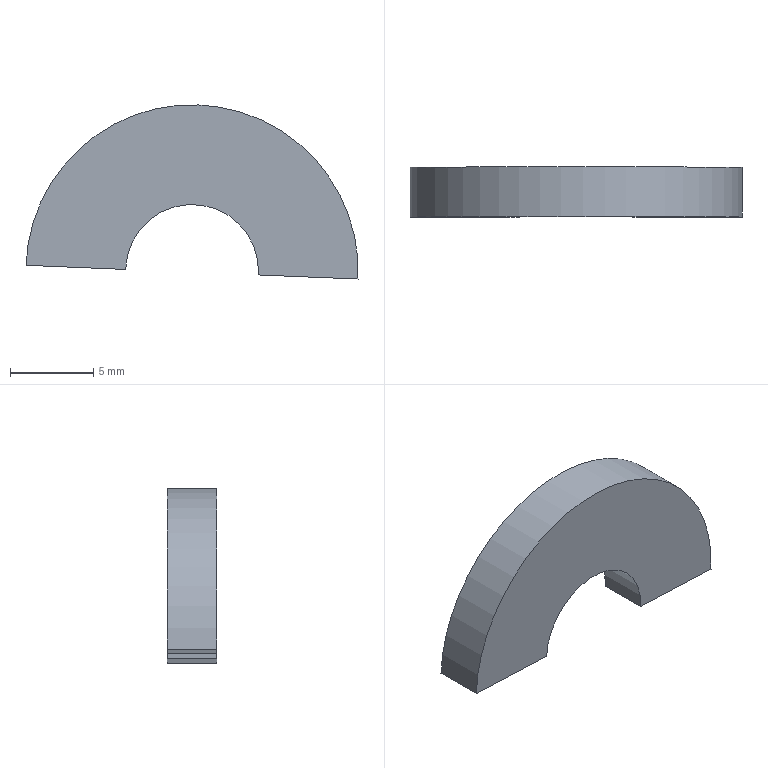Part | STEP file | Cuon T phu H01_8 | 1 solid | 6 faces | box 19.994 x 3 x 10.486 mm | volume 398.464 mm3 | plane 4 | cylinder 2 | commonest cylinder face diameters 8 x1 20 x1
STEP:
#1=CARTESIAN_POINT('',(0.,0.,0.));
#2=DIRECTION('',(0.,0.,1.));
#3=DIRECTION('',(1.,0.,0.));
#4=AXIS2_PLACEMENT_3D('',#1,#2,#3);
#5=CARTESIAN_POINT('',(-9.994,3.,0.3402));
#6=VERTEX_POINT('',#5);
#7=CARTESIAN_POINT('',(-3.999,3.,0.09239));
#8=VERTEX_POINT('',#7);
#9=CARTESIAN_POINT('',(-0.003009,3.,-0.0728));
#10=DIRECTION('',(0.9991,0.,-0.0413));
#11=VECTOR('',#10,1.);
#12=LINE('',#9,#11);
#13=CARTESIAN_POINT('',(0.,3.,0.));
#14=DIRECTION('',(0.,1.,0.));
#15=DIRECTION('',(0.,0.,1.));
#16=AXIS2_PLACEMENT_3D('',#13,#14,#15);
#17=PLANE('',#16);
#18=CARTESIAN_POINT('',(-0.0728,-0.003009));
#19=DIRECTION('',(-0.0413,0.9991));
#20=VECTOR('',#19,1.);
#21=LINE('',#18,#20);
#22=(GEOMETRIC_REPRESENTATION_CONTEXT(2)PARAMETRIC_REPRESENTATION_CONTEXT()REPRESENTATION_CONTEXT('',''));
#23=DEFINITIONAL_REPRESENTATION('',(#21),#22);
#24=PCURVE('',#17,#23);
#25=CARTESIAN_POINT('',(60.167,-18.57,-2.56));
#26=DIRECTION('',(0.0413,0.,0.9991));
#27=DIRECTION('',(0.9991,0.,-0.0413));
#28=AXIS2_PLACEMENT_3D('',#25,#26,#27);
#29=PLANE('',#28);
#30=CARTESIAN_POINT('',(-60.221,21.57));
#31=DIRECTION('',(1.,0.));
#32=VECTOR('',#31,1.);
#33=LINE('',#30,#32);
#34=(GEOMETRIC_REPRESENTATION_CONTEXT(2)PARAMETRIC_REPRESENTATION_CONTEXT()REPRESENTATION_CONTEXT('',''));
#35=DEFINITIONAL_REPRESENTATION('',(#33),#34);
#36=PCURVE('',#29,#35);
#37=SURFACE_CURVE('',#12,(#24,#36),.PCURVE_S1.);
#38=EDGE_CURVE('',#6,#8,#37,.T.);
#39=ORIENTED_EDGE('',*,*,#38,.F.);
#40=CARTESIAN_POINT('',(9.988,3.,-0.4858));
#41=VERTEX_POINT('',#40);
#42=CARTESIAN_POINT('',(0.,3.,0.));
#43=DIRECTION('',(0.,1.,0.));
#44=DIRECTION('',(0.,0.,1.));
#45=AXIS2_PLACEMENT_3D('',#42,#43,#44);
#46=CIRCLE('',#45,10.);
#47=CARTESIAN_POINT('',(0.,0.));
#48=DIRECTION('',(1.,0.));
#49=AXIS2_PLACEMENT_2D('',#47,#48);
#50=CIRCLE('',#49,10.);
#51=(GEOMETRIC_REPRESENTATION_CONTEXT(2)PARAMETRIC_REPRESENTATION_CONTEXT()REPRESENTATION_CONTEXT('',''));
#52=DEFINITIONAL_REPRESENTATION('',(#50),#51);
#53=PCURVE('',#17,#52);
#54=CARTESIAN_POINT('',(0.,3.,0.));
#55=DIRECTION('',(0.,-1.,0.));
#56=DIRECTION('',(0.,0.,-1.));
#57=AXIS2_PLACEMENT_3D('',#54,#55,#56);
#58=CYLINDRICAL_SURFACE('',#57,10.);
#59=CARTESIAN_POINT('',(9.425,0.));
#60=DIRECTION('',(-1.,0.));
#61=VECTOR('',#60,1.);
#62=LINE('',#59,#61);
#63=(GEOMETRIC_REPRESENTATION_CONTEXT(2)PARAMETRIC_REPRESENTATION_CONTEXT()REPRESENTATION_CONTEXT('',''));
#64=DEFINITIONAL_REPRESENTATION('',(#62),#63);
#65=PCURVE('',#58,#64);
#66=SURFACE_CURVE('',#46,(#53,#65),.PCURVE_S1.);
#67=EDGE_CURVE('',#6,#41,#66,.T.);
#68=ORIENTED_EDGE('',*,*,#67,.T.);
#69=CARTESIAN_POINT('',(3.993,3.,-0.238));
#70=VERTEX_POINT('',#69);
#71=CARTESIAN_POINT('',(-0.003009,3.,-0.0728));
#72=DIRECTION('',(0.9991,0.,-0.0413));
#73=VECTOR('',#72,1.);
#74=LINE('',#71,#73);
#75=CARTESIAN_POINT('',(-0.0728,-0.003009));
#76=DIRECTION('',(-0.0413,0.9991));
#77=VECTOR('',#76,1.);
#78=LINE('',#75,#77);
#79=(GEOMETRIC_REPRESENTATION_CONTEXT(2)PARAMETRIC_REPRESENTATION_CONTEXT()REPRESENTATION_CONTEXT('',''));
#80=DEFINITIONAL_REPRESENTATION('',(#78),#79);
#81=PCURVE('',#17,#80);
#82=CARTESIAN_POINT('',(60.167,-18.57,-2.56));
#83=DIRECTION('',(0.0413,0.,0.9991));
#84=DIRECTION('',(0.9991,0.,-0.0413));
#85=AXIS2_PLACEMENT_3D('',#82,#83,#84);
#86=PLANE('',#85);
#87=CARTESIAN_POINT('',(-60.221,21.57));
#88=DIRECTION('',(1.,0.));
#89=VECTOR('',#88,1.);
#90=LINE('',#87,#89);
#91=(GEOMETRIC_REPRESENTATION_CONTEXT(2)PARAMETRIC_REPRESENTATION_CONTEXT()REPRESENTATION_CONTEXT('',''));
#92=DEFINITIONAL_REPRESENTATION('',(#90),#91);
#93=PCURVE('',#86,#92);
#94=SURFACE_CURVE('',#74,(#81,#93),.PCURVE_S1.);
#95=EDGE_CURVE('',#70,#41,#94,.T.);
#96=ORIENTED_EDGE('',*,*,#95,.F.);
#97=CARTESIAN_POINT('',(0.,3.,0.));
#98=DIRECTION('',(0.,1.,0.));
#99=DIRECTION('',(0.,0.,1.));
#100=AXIS2_PLACEMENT_3D('',#97,#98,#99);
#101=CIRCLE('',#100,4.);
#102=CARTESIAN_POINT('',(0.,0.));
#103=DIRECTION('',(1.,0.));
#104=AXIS2_PLACEMENT_2D('',#102,#103);
#105=CIRCLE('',#104,4.);
#106=(GEOMETRIC_REPRESENTATION_CONTEXT(2)PARAMETRIC_REPRESENTATION_CONTEXT()REPRESENTATION_CONTEXT('',''));
#107=DEFINITIONAL_REPRESENTATION('',(#105),#106);
#108=PCURVE('',#17,#107);
#109=CARTESIAN_POINT('',(0.,3.,0.));
#110=DIRECTION('',(0.,-1.,0.));
#111=DIRECTION('',(0.,0.,-1.));
#112=AXIS2_PLACEMENT_3D('',#109,#110,#111);
#113=CYLINDRICAL_SURFACE('',#112,4.);
#114=CARTESIAN_POINT('',(9.425,0.));
#115=DIRECTION('',(-1.,0.));
#116=VECTOR('',#115,1.);
#117=LINE('',#114,#116);
#118=(GEOMETRIC_REPRESENTATION_CONTEXT(2)PARAMETRIC_REPRESENTATION_CONTEXT()REPRESENTATION_CONTEXT('',''));
#119=DEFINITIONAL_REPRESENTATION('',(#117),#118);
#120=PCURVE('',#113,#119);
#121=SURFACE_CURVE('',#101,(#108,#120),.PCURVE_S1.);
#122=EDGE_CURVE('',#8,#70,#121,.T.);
#123=ORIENTED_EDGE('',*,*,#122,.F.);
#124=EDGE_LOOP('',(#39,#68,#96,#123));
#125=FACE_BOUND('',#124,.T.);
#126=ADVANCED_FACE('',(#125),#17,.T.);
#127=CARTESIAN_POINT('',(-9.994,0.,0.3402));
#128=VERTEX_POINT('',#127);
#129=CARTESIAN_POINT('',(9.988,0.,-0.4858));
#130=VERTEX_POINT('',#129);
#131=CARTESIAN_POINT('',(0.,0.,0.));
#132=DIRECTION('',(0.,1.,0.));
#133=DIRECTION('',(0.,0.,1.));
#134=AXIS2_PLACEMENT_3D('',#131,#132,#133);
#135=CIRCLE('',#134,10.);
#136=CARTESIAN_POINT('',(0.,0.,0.));
#137=DIRECTION('',(0.,1.,0.));
#138=DIRECTION('',(0.,0.,1.));
#139=AXIS2_PLACEMENT_3D('',#136,#137,#138);
#140=PLANE('',#139);
#141=CARTESIAN_POINT('',(0.,0.));
#142=DIRECTION('',(1.,0.));
#143=AXIS2_PLACEMENT_2D('',#141,#142);
#144=CIRCLE('',#143,10.);
#145=(GEOMETRIC_REPRESENTATION_CONTEXT(2)PARAMETRIC_REPRESENTATION_CONTEXT()REPRESENTATION_CONTEXT('',''));
#146=DEFINITIONAL_REPRESENTATION('',(#144),#145);
#147=PCURVE('',#140,#146);
#148=CARTESIAN_POINT('',(9.425,3.));
#149=DIRECTION('',(-1.,0.));
#150=VECTOR('',#149,1.);
#151=LINE('',#148,#150);
#152=(GEOMETRIC_REPRESENTATION_CONTEXT(2)PARAMETRIC_REPRESENTATION_CONTEXT()REPRESENTATION_CONTEXT('',''));
#153=DEFINITIONAL_REPRESENTATION('',(#151),#152);
#154=PCURVE('',#58,#153);
#155=SURFACE_CURVE('',#135,(#147,#154),.PCURVE_S1.);
#156=EDGE_CURVE('',#128,#130,#155,.T.);
#157=ORIENTED_EDGE('',*,*,#156,.F.);
#158=CARTESIAN_POINT('',(-3.999,0.,0.09239));
#159=VERTEX_POINT('',#158);
#160=CARTESIAN_POINT('',(-0.003009,0.,-0.0728));
#161=DIRECTION('',(0.9991,0.,-0.0413));
#162=VECTOR('',#161,1.);
#163=LINE('',#160,#162);
#164=CARTESIAN_POINT('',(-0.0728,-0.003009));
#165=DIRECTION('',(-0.0413,0.9991));
#166=VECTOR('',#165,1.);
#167=LINE('',#164,#166);
#168=(GEOMETRIC_REPRESENTATION_CONTEXT(2)PARAMETRIC_REPRESENTATION_CONTEXT()REPRESENTATION_CONTEXT('',''));
#169=DEFINITIONAL_REPRESENTATION('',(#167),#168);
#170=PCURVE('',#140,#169);
#171=CARTESIAN_POINT('',(-60.221,18.57));
#172=DIRECTION('',(1.,0.));
#173=VECTOR('',#172,1.);
#174=LINE('',#171,#173);
#175=(GEOMETRIC_REPRESENTATION_CONTEXT(2)PARAMETRIC_REPRESENTATION_CONTEXT()REPRESENTATION_CONTEXT('',''));
#176=DEFINITIONAL_REPRESENTATION('',(#174),#175);
#177=PCURVE('',#29,#176);
#178=SURFACE_CURVE('',#163,(#170,#177),.PCURVE_S1.);
#179=EDGE_CURVE('',#128,#159,#178,.T.);
#180=ORIENTED_EDGE('',*,*,#179,.T.);
#181=CARTESIAN_POINT('',(3.993,0.,-0.238));
#182=VERTEX_POINT('',#181);
#183=CARTESIAN_POINT('',(0.,0.,0.));
#184=DIRECTION('',(0.,1.,0.));
#185=DIRECTION('',(0.,0.,1.));
#186=AXIS2_PLACEMENT_3D('',#183,#184,#185);
#187=CIRCLE('',#186,4.);
#188=CARTESIAN_POINT('',(0.,0.));
#189=DIRECTION('',(1.,0.));
#190=AXIS2_PLACEMENT_2D('',#188,#189);
#191=CIRCLE('',#190,4.);
#192=(GEOMETRIC_REPRESENTATION_CONTEXT(2)PARAMETRIC_REPRESENTATION_CONTEXT()REPRESENTATION_CONTEXT('',''));
#193=DEFINITIONAL_REPRESENTATION('',(#191),#192);
#194=PCURVE('',#140,#193);
#195=CARTESIAN_POINT('',(9.425,3.));
#196=DIRECTION('',(-1.,0.));
#197=VECTOR('',#196,1.);
#198=LINE('',#195,#197);
#199=(GEOMETRIC_REPRESENTATION_CONTEXT(2)PARAMETRIC_REPRESENTATION_CONTEXT()REPRESENTATION_CONTEXT('',''));
#200=DEFINITIONAL_REPRESENTATION('',(#198),#199);
#201=PCURVE('',#113,#200);
#202=SURFACE_CURVE('',#187,(#194,#201),.PCURVE_S1.);
#203=EDGE_CURVE('',#159,#182,#202,.T.);
#204=ORIENTED_EDGE('',*,*,#203,.T.);
#205=CARTESIAN_POINT('',(-0.003009,0.,-0.0728));
#206=DIRECTION('',(0.9991,0.,-0.0413));
#207=VECTOR('',#206,1.);
#208=LINE('',#205,#207);
#209=CARTESIAN_POINT('',(-0.0728,-0.003009));
#210=DIRECTION('',(-0.0413,0.9991));
#211=VECTOR('',#210,1.);
#212=LINE('',#209,#211);
#213=(GEOMETRIC_REPRESENTATION_CONTEXT(2)PARAMETRIC_REPRESENTATION_CONTEXT()REPRESENTATION_CONTEXT('',''));
#214=DEFINITIONAL_REPRESENTATION('',(#212),#213);
#215=PCURVE('',#140,#214);
#216=CARTESIAN_POINT('',(-60.221,18.57));
#217=DIRECTION('',(1.,0.));
#218=VECTOR('',#217,1.);
#219=LINE('',#216,#218);
#220=(GEOMETRIC_REPRESENTATION_CONTEXT(2)PARAMETRIC_REPRESENTATION_CONTEXT()REPRESENTATION_CONTEXT('',''));
#221=DEFINITIONAL_REPRESENTATION('',(#219),#220);
#222=PCURVE('',#86,#221);
#223=SURFACE_CURVE('',#208,(#215,#222),.PCURVE_S1.);
#224=EDGE_CURVE('',#182,#130,#223,.T.);
#225=ORIENTED_EDGE('',*,*,#224,.T.);
#226=EDGE_LOOP('',(#157,#180,#204,#225));
#227=FACE_BOUND('',#226,.T.);
#228=ADVANCED_FACE('',(#227),#140,.F.);
#229=ORIENTED_EDGE('',*,*,#67,.F.);
#230=CARTESIAN_POINT('',(-9.994,3.,0.3402));
#231=DIRECTION('',(0.,-1.,0.));
#232=VECTOR('',#231,1.);
#233=LINE('',#230,#232);
#234=CARTESIAN_POINT('',(4.678,0.));
#235=DIRECTION('',(0.,1.));
#236=VECTOR('',#235,1.);
#237=LINE('',#234,#236);
#238=(GEOMETRIC_REPRESENTATION_CONTEXT(2)PARAMETRIC_REPRESENTATION_CONTEXT()REPRESENTATION_CONTEXT('',''));
#239=DEFINITIONAL_REPRESENTATION('',(#237),#238);
#240=PCURVE('',#58,#239);
#241=CARTESIAN_POINT('',(-70.221,21.57));
#242=DIRECTION('',(0.,-1.));
#243=VECTOR('',#242,1.);
#244=LINE('',#241,#243);
#245=(GEOMETRIC_REPRESENTATION_CONTEXT(2)PARAMETRIC_REPRESENTATION_CONTEXT()REPRESENTATION_CONTEXT('',''));
#246=DEFINITIONAL_REPRESENTATION('',(#244),#245);
#247=PCURVE('',#29,#246);
#248=SURFACE_CURVE('',#233,(#240,#247),.PCURVE_S1.);
#249=EDGE_CURVE('',#6,#128,#248,.T.);
#250=ORIENTED_EDGE('',*,*,#249,.T.);
#251=ORIENTED_EDGE('',*,*,#156,.T.);
#252=CARTESIAN_POINT('',(9.988,3.,-0.4858));
#253=DIRECTION('',(0.,1.,0.));
#254=VECTOR('',#253,1.);
#255=LINE('',#252,#254);
#256=CARTESIAN_POINT('',(1.522,0.));
#257=DIRECTION('',(0.,-1.));
#258=VECTOR('',#257,1.);
#259=LINE('',#256,#258);
#260=(GEOMETRIC_REPRESENTATION_CONTEXT(2)PARAMETRIC_REPRESENTATION_CONTEXT()REPRESENTATION_CONTEXT('',''));
#261=DEFINITIONAL_REPRESENTATION('',(#259),#260);
#262=PCURVE('',#58,#261);
#263=CARTESIAN_POINT('',(-50.222,21.57));
#264=DIRECTION('',(0.,1.));
#265=VECTOR('',#264,1.);
#266=LINE('',#263,#265);
#267=(GEOMETRIC_REPRESENTATION_CONTEXT(2)PARAMETRIC_REPRESENTATION_CONTEXT()REPRESENTATION_CONTEXT('',''));
#268=DEFINITIONAL_REPRESENTATION('',(#266),#267);
#269=PCURVE('',#86,#268);
#270=SURFACE_CURVE('',#255,(#262,#269),.PCURVE_S1.);
#271=EDGE_CURVE('',#130,#41,#270,.T.);
#272=ORIENTED_EDGE('',*,*,#271,.T.);
#273=EDGE_LOOP('',(#229,#250,#251,#272));
#274=FACE_BOUND('',#273,.T.);
#275=ADVANCED_FACE('',(#274),#58,.T.);
#276=ORIENTED_EDGE('',*,*,#203,.T.);
#277=CARTESIAN_POINT('',(3.993,3.,-0.238));
#278=DIRECTION('',(0.,1.,0.));
#279=VECTOR('',#278,1.);
#280=LINE('',#277,#279);
#281=CARTESIAN_POINT('',(1.511,0.));
#282=DIRECTION('',(0.,-1.));
#283=VECTOR('',#282,1.);
#284=LINE('',#281,#283);
#285=(GEOMETRIC_REPRESENTATION_CONTEXT(2)PARAMETRIC_REPRESENTATION_CONTEXT()REPRESENTATION_CONTEXT('',''));
#286=DEFINITIONAL_REPRESENTATION('',(#284),#285);
#287=PCURVE('',#113,#286);
#288=CARTESIAN_POINT('',(-56.222,21.57));
#289=DIRECTION('',(0.,1.));
#290=VECTOR('',#289,1.);
#291=LINE('',#288,#290);
#292=(GEOMETRIC_REPRESENTATION_CONTEXT(2)PARAMETRIC_REPRESENTATION_CONTEXT()REPRESENTATION_CONTEXT('',''));
#293=DEFINITIONAL_REPRESENTATION('',(#291),#292);
#294=PCURVE('',#86,#293);
#295=SURFACE_CURVE('',#280,(#287,#294),.PCURVE_S1.);
#296=EDGE_CURVE('',#182,#70,#295,.T.);
#297=ORIENTED_EDGE('',*,*,#296,.T.);
#298=ORIENTED_EDGE('',*,*,#122,.F.);
#299=CARTESIAN_POINT('',(-3.999,3.,0.09239));
#300=DIRECTION('',(0.,-1.,0.));
#301=VECTOR('',#300,1.);
#302=LINE('',#299,#301);
#303=CARTESIAN_POINT('',(4.689,0.));
#304=DIRECTION('',(0.,1.));
#305=VECTOR('',#304,1.);
#306=LINE('',#303,#305);
#307=(GEOMETRIC_REPRESENTATION_CONTEXT(2)PARAMETRIC_REPRESENTATION_CONTEXT()REPRESENTATION_CONTEXT('',''));
#308=DEFINITIONAL_REPRESENTATION('',(#306),#307);
#309=PCURVE('',#113,#308);
#310=CARTESIAN_POINT('',(-64.221,21.57));
#311=DIRECTION('',(0.,-1.));
#312=VECTOR('',#311,1.);
#313=LINE('',#310,#312);
#314=(GEOMETRIC_REPRESENTATION_CONTEXT(2)PARAMETRIC_REPRESENTATION_CONTEXT()REPRESENTATION_CONTEXT('',''));
#315=DEFINITIONAL_REPRESENTATION('',(#313),#314);
#316=PCURVE('',#29,#315);
#317=SURFACE_CURVE('',#302,(#309,#316),.PCURVE_S1.);
#318=EDGE_CURVE('',#8,#159,#317,.T.);
#319=ORIENTED_EDGE('',*,*,#318,.T.);
#320=EDGE_LOOP('',(#276,#297,#298,#319));
#321=FACE_BOUND('',#320,.F.);
#322=ADVANCED_FACE('',(#321),#113,.F.);
#323=ORIENTED_EDGE('',*,*,#224,.F.);
#324=ORIENTED_EDGE('',*,*,#296,.T.);
#325=ORIENTED_EDGE('',*,*,#95,.T.);
#326=ORIENTED_EDGE('',*,*,#271,.F.);
#327=EDGE_LOOP('',(#323,#324,#325,#326));
#328=FACE_BOUND('',#327,.T.);
#329=ADVANCED_FACE('',(#328),#86,.F.);
#330=ORIENTED_EDGE('',*,*,#38,.T.);
#331=ORIENTED_EDGE('',*,*,#318,.T.);
#332=ORIENTED_EDGE('',*,*,#179,.F.);
#333=ORIENTED_EDGE('',*,*,#249,.F.);
#334=EDGE_LOOP('',(#330,#331,#332,#333));
#335=FACE_BOUND('',#334,.T.);
#336=ADVANCED_FACE('',(#335),#29,.F.);
#337=CLOSED_SHELL('',(#126,#228,#275,#322,#329,#336));
#338=MANIFOLD_SOLID_BREP('',#337);
#339=(LENGTH_UNIT()NAMED_UNIT(*)SI_UNIT(.MILLI.,.METRE.));
#340=UNCERTAINTY_MEASURE_WITH_UNIT(LENGTH_MEASURE(0.0000001),#339,'','');
#341=(NAMED_UNIT(*)PLANE_ANGLE_UNIT()SI_UNIT($,.RADIAN.));
#342=(NAMED_UNIT(*)SI_UNIT($,.STERADIAN.)SOLID_ANGLE_UNIT());
#343=(GEOMETRIC_REPRESENTATION_CONTEXT(3)GLOBAL_UNCERTAINTY_ASSIGNED_CONTEXT((#340))GLOBAL_UNIT_ASSIGNED_CONTEXT((#339,#341,#342))REPRESENTATION_CONTEXT('',''));
#344=ADVANCED_BREP_SHAPE_REPRESENTATION('',(#4,#338),#343);